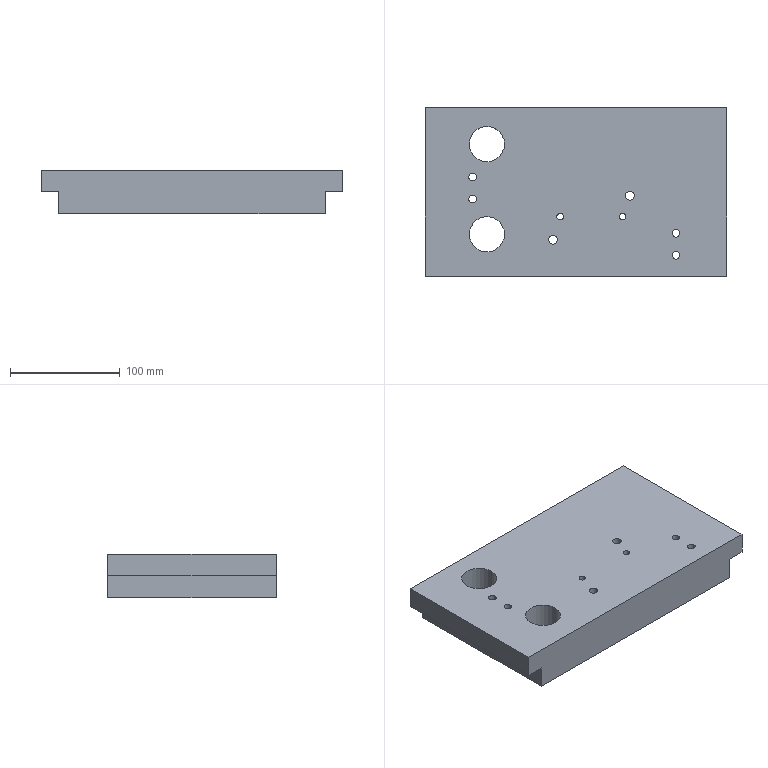Part | 1 solid | 61 faces | box 273.935 x 153 x 40 mm | volume 1342014 mm3 | cylinder 36 | plane 17 | cone 8 | commonest cylinder face diameters 8 x12 7 x8 6 x4 10 x4 32 x4 34 x4